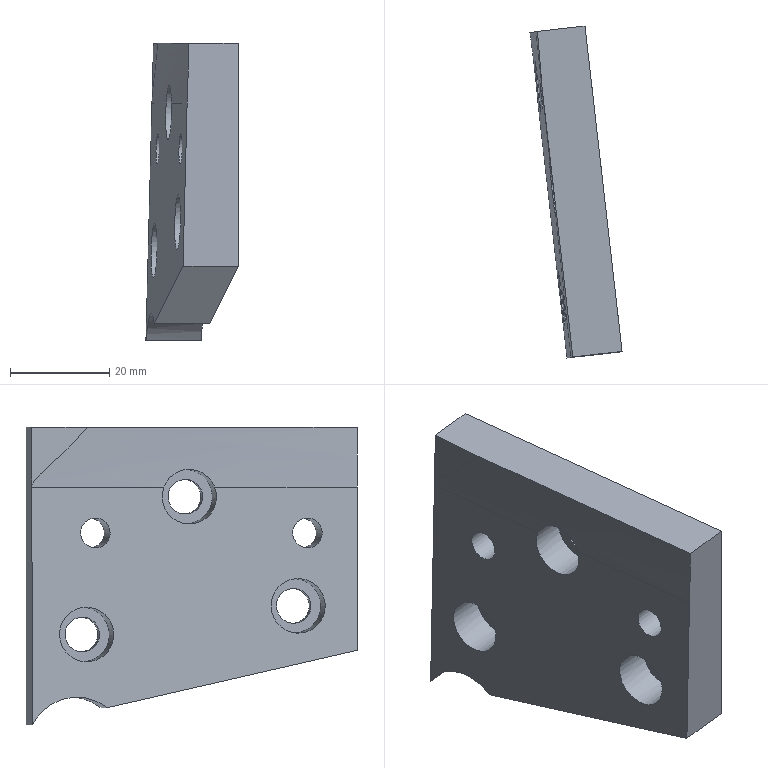Part | NX | features XQ 2 | 1 solid | 21 faces | box 18.578 x 66.841 x 59.998 mm | volume 32864 mm3 | plane 11 | cylinder 9 | spline 1 | commonest cylinder face diameters 7 x3 11 x3 6.001 x2 20 x1
STEP:
#1=CARTESIAN_POINT('',(2664.559,193.904,-66.597));
#2=VERTEX_POINT('',#1);
#3=CARTESIAN_POINT('',(2664.604,193.511,-63.12));
#4=DIRECTION('',(-0.9936,-0.1132,0.));
#5=DIRECTION('',(-0.01281,0.1125,-0.9936));
#6=AXIS2_PLACEMENT_3D('',#3,#4,#5);
#7=CIRCLE('',#6,3.5);
#8=EDGE_CURVE('',#2,#2,#7,.T.);
#9=ORIENTED_EDGE('',*,*,#8,.F.);
#10=EDGE_LOOP('',(#9));
#11=FACE_BOUND('',#10,.T.);
#12=CARTESIAN_POINT('',(2664.674,192.892,-57.655));
#13=VERTEX_POINT('',#12);
#14=CARTESIAN_POINT('',(2664.604,193.511,-63.12));
#15=DIRECTION('',(-0.9936,-0.1132,0.));
#16=DIRECTION('',(0.01281,-0.1125,0.9936));
#17=AXIS2_PLACEMENT_3D('',#14,#15,#16);
#18=CIRCLE('',#17,5.5);
#19=EDGE_CURVE('',#13,#13,#18,.T.);
#20=ORIENTED_EDGE('',*,*,#19,.T.);
#21=EDGE_LOOP('',(#20));
#22=FACE_BOUND('',#21,.T.);
#23=CARTESIAN_POINT('',(2664.604,193.511,-63.12));
#24=DIRECTION('',(0.9936,0.1132,0.));
#25=DIRECTION('',(0.01281,-0.1125,0.9936));
#26=AXIS2_PLACEMENT_3D('',#23,#24,#25);
#27=PLANE('',#26);
#28=ADVANCED_FACE('',(#11,#22),#27,.F.);
#29=CARTESIAN_POINT('',(2659.703,236.529,-72.371));
#30=VERTEX_POINT('',#29);
#31=CARTESIAN_POINT('',(2659.747,236.136,-68.894));
#32=DIRECTION('',(-0.9936,-0.1132,0.));
#33=DIRECTION('',(-0.01281,0.1125,-0.9936));
#34=AXIS2_PLACEMENT_3D('',#31,#32,#33);
#35=CIRCLE('',#34,3.5);
#36=EDGE_CURVE('',#30,#30,#35,.T.);
#37=ORIENTED_EDGE('',*,*,#36,.F.);
#38=EDGE_LOOP('',(#37));
#39=FACE_BOUND('',#38,.T.);
#40=CARTESIAN_POINT('',(2659.818,235.517,-63.429));
#41=VERTEX_POINT('',#40);
#42=CARTESIAN_POINT('',(2659.747,236.136,-68.894));
#43=DIRECTION('',(-0.9936,-0.1132,0.));
#44=DIRECTION('',(0.01281,-0.1125,0.9936));
#45=AXIS2_PLACEMENT_3D('',#42,#43,#44);
#46=CIRCLE('',#45,5.5);
#47=EDGE_CURVE('',#41,#41,#46,.T.);
#48=ORIENTED_EDGE('',*,*,#47,.T.);
#49=EDGE_LOOP('',(#48));
#50=FACE_BOUND('',#49,.T.);
#51=CARTESIAN_POINT('',(2659.747,236.136,-68.894));
#52=DIRECTION('',(0.9936,0.1132,0.));
#53=DIRECTION('',(0.01281,-0.1125,0.9936));
#54=AXIS2_PLACEMENT_3D('',#51,#52,#53);
#55=PLANE('',#54);
#56=ADVANCED_FACE('',(#39,#50),#55,.F.);
#57=CARTESIAN_POINT('',(2662.184,214.751,-35.655));
#58=VERTEX_POINT('',#57);
#59=CARTESIAN_POINT('',(2662.113,215.369,-41.12));
#60=DIRECTION('',(-0.9936,-0.1132,0.));
#61=DIRECTION('',(0.01281,-0.1125,0.9936));
#62=AXIS2_PLACEMENT_3D('',#59,#60,#61);
#63=CIRCLE('',#62,5.5);
#64=EDGE_CURVE('',#58,#58,#63,.T.);
#65=ORIENTED_EDGE('',*,*,#64,.T.);
#66=EDGE_LOOP('',(#65));
#67=FACE_BOUND('',#66,.T.);
#68=CARTESIAN_POINT('',(2662.069,215.763,-44.597));
#69=VERTEX_POINT('',#68);
#70=CARTESIAN_POINT('',(2662.113,215.369,-41.12));
#71=DIRECTION('',(-0.9936,-0.1132,0.));
#72=DIRECTION('',(-0.01281,0.1125,-0.9936));
#73=AXIS2_PLACEMENT_3D('',#70,#71,#72);
#74=CIRCLE('',#73,3.5);
#75=EDGE_CURVE('',#69,#69,#74,.T.);
#76=ORIENTED_EDGE('',*,*,#75,.F.);
#77=EDGE_LOOP('',(#76));
#78=FACE_BOUND('',#77,.T.);
#79=CARTESIAN_POINT('',(2662.113,215.369,-41.12));
#80=DIRECTION('',(0.9936,0.1132,0.));
#81=DIRECTION('',(0.01281,-0.1125,0.9936));
#82=AXIS2_PLACEMENT_3D('',#79,#80,#81);
#83=PLANE('',#82);
#84=ADVANCED_FACE('',(#67,#78),#83,.F.);
#85=ORIENTED_EDGE('',*,*,#19,.F.);
#86=EDGE_LOOP('',(#85));
#87=FACE_BOUND('',#86,.T.);
#88=CARTESIAN_POINT('',(2656.779,193.849,-57.757));
#89=VERTEX_POINT('',#88);
#90=CARTESIAN_POINT('',(2656.775,192.619,-63.12));
#91=DIRECTION('',(-0.9939,-0.1074,0.02552));
#92=DIRECTION('',(0.0008715,0.2236,0.9747));
#93=AXIS2_PLACEMENT_3D('',#90,#91,#92);
#94=ELLIPSE('',#93,5.502,5.5);
#95=EDGE_CURVE('',#89,#89,#94,.T.);
#96=ORIENTED_EDGE('',*,*,#95,.T.);
#97=EDGE_LOOP('',(#96));
#98=FACE_BOUND('',#97,.T.);
#99=CARTESIAN_POINT('',(2657.649,192.718,-63.12));
#100=DIRECTION('',(0.9936,0.1132,0.));
#101=DIRECTION('',(-0.01281,0.1125,-0.9936));
#102=AXIS2_PLACEMENT_3D('',#99,#100,#101);
#103=CYLINDRICAL_SURFACE('',#102,5.5);
#104=ADVANCED_FACE('',(#87,#98),#103,.F.);
#105=CARTESIAN_POINT('',(2667.981,190.373,-63.12));
#106=VERTEX_POINT('',#105);
#107=CARTESIAN_POINT('',(2667.585,193.85,-63.12));
#108=DIRECTION('',(-0.9936,-0.1132,-0.000000001));
#109=DIRECTION('',(0.1132,-0.9936,0.));
#110=AXIS2_PLACEMENT_3D('',#107,#108,#109);
#111=CIRCLE('',#110,3.5);
#112=EDGE_CURVE('',#106,#106,#111,.T.);
#113=ORIENTED_EDGE('',*,*,#112,.F.);
#114=EDGE_LOOP('',(#113));
#115=FACE_BOUND('',#114,.T.);
#116=ORIENTED_EDGE('',*,*,#8,.T.);
#117=EDGE_LOOP('',(#116));
#118=FACE_BOUND('',#117,.T.);
#119=CARTESIAN_POINT('',(2655.662,192.492,-63.12));
#120=DIRECTION('',(0.9936,0.1132,0.));
#121=DIRECTION('',(-0.01281,0.1125,-0.9936));
#122=AXIS2_PLACEMENT_3D('',#119,#120,#121);
#123=CYLINDRICAL_SURFACE('',#122,3.5);
#124=ADVANCED_FACE('',(#115,#118),#123,.F.);
#125=CARTESIAN_POINT('',(2668.142,188.959,-48.416));
#126=VERTEX_POINT('',#125);
#127=CARTESIAN_POINT('',(2667.802,191.94,-48.416));
#128=DIRECTION('',(-0.9936,-0.1132,-0.000000001));
#129=DIRECTION('',(0.1132,-0.9936,0.));
#130=AXIS2_PLACEMENT_3D('',#127,#128,#129);
#131=CIRCLE('',#130,3.001);
#132=EDGE_CURVE('',#126,#126,#131,.T.);
#133=ORIENTED_EDGE('',*,*,#132,.F.);
#134=EDGE_LOOP('',(#133));
#135=FACE_BOUND('',#134,.T.);
#136=CARTESIAN_POINT('',(2657.357,191.421,-45.49));
#137=VERTEX_POINT('',#136);
#138=CARTESIAN_POINT('',(2657.354,190.75,-48.416));
#139=DIRECTION('',(-0.9939,-0.1074,0.02552));
#140=DIRECTION('',(0.0008715,0.2236,0.9747));
#141=AXIS2_PLACEMENT_3D('',#138,#139,#140);
#142=ELLIPSE('',#141,3.002,3.001);
#143=EDGE_CURVE('',#137,#137,#142,.T.);
#144=ORIENTED_EDGE('',*,*,#143,.T.);
#145=EDGE_LOOP('',(#144));
#146=FACE_BOUND('',#145,.T.);
#147=CARTESIAN_POINT('',(2655.879,190.582,-48.416));
#148=DIRECTION('',(0.9936,0.1132,0.));
#149=DIRECTION('',(-0.01281,0.1125,-0.9936));
#150=AXIS2_PLACEMENT_3D('',#147,#148,#149);
#151=CYLINDRICAL_SURFACE('',#150,3.001);
#152=ADVANCED_FACE('',(#135,#146),#151,.F.);
#153=CARTESIAN_POINT('',(2658.679,180.692,-39.162));
#154=VERTEX_POINT('',#153);
#155=CARTESIAN_POINT('',(2657.844,180.597,-72.062));
#156=VERTEX_POINT('',#155);
#157=CARTESIAN_POINT('',(2659.681,180.806,0.3658));
#158=DIRECTION('',(-0.02536,-0.002889,-0.9997));
#159=VECTOR('',#158,1000.);
#160=LINE('',#157,#159);
#161=EDGE_CURVE('',#154,#156,#160,.T.);
#162=ORIENTED_EDGE('',*,*,#161,.T.);
#163=CARTESIAN_POINT('',(2668.95,181.863,-72.062));
#164=VERTEX_POINT('',#163);
#165=CARTESIAN_POINT('',(2673.918,182.429,-72.062));
#166=DIRECTION('',(-0.9936,-0.1132,-0.000000001));
#167=VECTOR('',#166,1000.);
#168=LINE('',#165,#167);
#169=EDGE_CURVE('',#164,#156,#168,.T.);
#170=ORIENTED_EDGE('',*,*,#169,.F.);
#171=CARTESIAN_POINT('',(2668.95,181.863,-27.1));
#172=VERTEX_POINT('',#171);
#173=CARTESIAN_POINT('',(2668.95,181.863,-0.000000058));
#174=DIRECTION('',(0.000000001,0.,-1.));
#175=VECTOR('',#174,1000.);
#176=LINE('',#173,#175);
#177=EDGE_CURVE('',#172,#164,#176,.T.);
#178=ORIENTED_EDGE('',*,*,#177,.F.);
#179=CARTESIAN_POINT('',(2659.015,180.73,-27.1));
#180=VERTEX_POINT('',#179);
#181=CARTESIAN_POINT('',(2673.918,182.429,-27.1));
#182=DIRECTION('',(0.9936,0.1132,0.));
#183=VECTOR('',#182,1000.);
#184=LINE('',#181,#183);
#185=EDGE_CURVE('',#180,#172,#184,.T.);
#186=ORIENTED_EDGE('',*,*,#185,.F.);
#187=CARTESIAN_POINT('',(2659.015,180.73,-27.1));
#188=CARTESIAN_POINT('',(2659.015,180.73,-31.123));
#189=CARTESIAN_POINT('',(2658.781,180.704,-35.141));
#190=CARTESIAN_POINT('',(2658.679,180.692,-39.162));
#191=B_SPLINE_CURVE_WITH_KNOTS('',3,(#187,#188,#189,#190),.UNSPECIFIED.,.F.,.F.,(4,4),(0.,0.01207),.UNSPECIFIED.);
#192=EDGE_CURVE('',#180,#154,#191,.T.);
#193=ORIENTED_EDGE('',*,*,#192,.T.);
#194=EDGE_LOOP('',(#162,#170,#178,#186,#193));
#195=FACE_BOUND('',#194,.T.);
#196=CARTESIAN_POINT('',(2673.918,182.429,-0.000000058));
#197=DIRECTION('',(0.1132,-0.9936,0.));
#198=DIRECTION('',(0.9936,0.1132,0.));
#199=AXIS2_PLACEMENT_3D('',#196,#197,#198);
#200=PLANE('',#199);
#201=ADVANCED_FACE('',(#195),#200,.T.);
#202=CARTESIAN_POINT('',(2652.091,231.089,-83.639));
#203=VERTEX_POINT('',#202);
#204=CARTESIAN_POINT('',(2663.198,232.355,-83.639));
#205=VERTEX_POINT('',#204);
#206=CARTESIAN_POINT('',(3040.755,275.372,-83.639));
#207=DIRECTION('',(0.9936,0.1132,0.000000001));
#208=VECTOR('',#207,1000.);
#209=LINE('',#206,#208);
#210=EDGE_CURVE('',#203,#205,#209,.T.);
#211=ORIENTED_EDGE('',*,*,#210,.T.);
#212=CARTESIAN_POINT('',(2503.911,1630.398,-404.205));
#213=DIRECTION('',(0.1104,-0.9687,0.2221));
#214=VECTOR('',#213,1000.);
#215=LINE('',#212,#214);
#216=EDGE_CURVE('',#205,#164,#215,.T.);
#217=ORIENTED_EDGE('',*,*,#216,.T.);
#218=ORIENTED_EDGE('',*,*,#169,.T.);
#219=CARTESIAN_POINT('',(2492.804,1629.133,-404.205));
#220=DIRECTION('',(0.1104,-0.9687,0.2221));
#221=VECTOR('',#220,1000.);
#222=LINE('',#219,#221);
#223=EDGE_CURVE('',#203,#156,#222,.T.);
#224=ORIENTED_EDGE('',*,*,#223,.F.);
#225=EDGE_LOOP('',(#211,#217,#218,#224));
#226=FACE_BOUND('',#225,.T.);
#227=CARTESIAN_POINT('',(2652.739,302.066,-99.689));
#228=DIRECTION('',(0.02515,-0.2207,-0.975));
#229=DIRECTION('',(0.,0.9753,-0.2208));
#230=AXIS2_PLACEMENT_3D('',#227,#228,#229);
#231=PLANE('',#230);
#232=ADVANCED_FACE('',(#226),#231,.T.);
#233=CARTESIAN_POINT('',(2661.482,247.415,-87.093));
#234=VERTEX_POINT('',#233);
#235=CARTESIAN_POINT('',(2662.498,238.496,-91.5));
#236=DIRECTION('',(-0.9936,-0.1132,-0.000000001));
#237=DIRECTION('',(0.000000001,0.,-1.));
#238=AXIS2_PLACEMENT_3D('',#235,#236,#237);
#239=CIRCLE('',#238,10.);
#240=EDGE_CURVE('',#205,#234,#239,.T.);
#241=ORIENTED_EDGE('',*,*,#240,.F.);
#242=ORIENTED_EDGE('',*,*,#210,.F.);
#243=CARTESIAN_POINT('',(2650.375,246.149,-87.093));
#244=VERTEX_POINT('',#243);
#245=CARTESIAN_POINT('',(2651.228,237.212,-91.5));
#246=DIRECTION('',(-0.9939,-0.1074,0.02552));
#247=DIRECTION('',(-0.0008715,-0.2236,-0.9747));
#248=AXIS2_PLACEMENT_3D('',#245,#246,#247);
#249=ELLIPSE('',#248,10.003,10.);
#250=EDGE_CURVE('',#203,#244,#249,.T.);
#251=ORIENTED_EDGE('',*,*,#250,.T.);
#252=CARTESIAN_POINT('',(3039.039,290.432,-87.093));
#253=DIRECTION('',(-0.9936,-0.1132,-0.000000001));
#254=VECTOR('',#253,1000.);
#255=LINE('',#252,#254);
#256=EDGE_CURVE('',#234,#244,#255,.T.);
#257=ORIENTED_EDGE('',*,*,#256,.F.);
#258=EDGE_LOOP('',(#241,#242,#251,#257));
#259=FACE_BOUND('',#258,.T.);
#260=CARTESIAN_POINT('',(3040.055,281.513,-91.5));
#261=DIRECTION('',(-0.9936,-0.1132,-0.000000001));
#262=DIRECTION('',(0.000000001,0.,-1.));
#263=AXIS2_PLACEMENT_3D('',#260,#261,#262);
#264=CYLINDRICAL_SURFACE('',#263,10.);
#265=ADVANCED_FACE('',(#259),#264,.F.);
#266=CARTESIAN_POINT('',(2650.373,246.173,-87.098));
#267=VERTEX_POINT('',#266);
#268=CARTESIAN_POINT('',(2661.479,247.438,-87.098));
#269=VERTEX_POINT('',#268);
#270=CARTESIAN_POINT('',(2658.995,247.155,-87.098));
#271=DIRECTION('',(0.9936,0.1132,0.000000001));
#272=VECTOR('',#271,1000.);
#273=LINE('',#270,#272);
#274=EDGE_CURVE('',#267,#269,#273,.T.);
#275=ORIENTED_EDGE('',*,*,#274,.T.);
#276=CARTESIAN_POINT('',(2503.911,1630.398,-404.205));
#277=DIRECTION('',(0.1104,-0.9687,0.2221));
#278=VECTOR('',#277,1000.);
#279=LINE('',#276,#278);
#280=EDGE_CURVE('',#269,#234,#279,.T.);
#281=ORIENTED_EDGE('',*,*,#280,.T.);
#282=ORIENTED_EDGE('',*,*,#256,.T.);
#283=CARTESIAN_POINT('',(2492.804,1629.133,-404.205));
#284=DIRECTION('',(0.1104,-0.9687,0.2221));
#285=VECTOR('',#284,1000.);
#286=LINE('',#283,#285);
#287=EDGE_CURVE('',#267,#244,#286,.T.);
#288=ORIENTED_EDGE('',*,*,#287,.F.);
#289=EDGE_LOOP('',(#275,#281,#282,#288));
#290=FACE_BOUND('',#289,.T.);
#291=CARTESIAN_POINT('',(2652.739,302.066,-99.689));
#292=DIRECTION('',(0.02515,-0.2207,-0.975));
#293=DIRECTION('',(0.,0.9753,-0.2208));
#294=AXIS2_PLACEMENT_3D('',#291,#292,#293);
#295=PLANE('',#294);
#296=ADVANCED_FACE('',(#290),#295,.T.);
#297=CARTESIAN_POINT('',(2651.895,246.346,-27.1));
#298=VERTEX_POINT('',#297);
#299=CARTESIAN_POINT('',(2651.593,246.312,-38.979));
#300=VERTEX_POINT('',#299);
#301=CARTESIAN_POINT('',(2651.895,246.346,-27.1));
#302=DIRECTION('',(-0.02539,-0.002893,-0.9997));
#303=VECTOR('',#302,1000.);
#304=LINE('',#301,#303);
#305=EDGE_CURVE('',#298,#300,#304,.T.);
#306=ORIENTED_EDGE('',*,*,#305,.F.);
#307=CARTESIAN_POINT('',(2661.479,247.438,-27.1));
#308=VERTEX_POINT('',#307);
#309=CARTESIAN_POINT('',(2651.543,246.306,-27.1));
#310=DIRECTION('',(0.9936,0.1132,0.));
#311=VECTOR('',#310,1000.);
#312=LINE('',#309,#311);
#313=EDGE_CURVE('',#298,#308,#312,.T.);
#314=ORIENTED_EDGE('',*,*,#313,.T.);
#315=CARTESIAN_POINT('',(2661.479,247.438,-706.6));
#316=DIRECTION('',(0.000000001,0.,-1.));
#317=VECTOR('',#316,1000.);
#318=LINE('',#315,#317);
#319=EDGE_CURVE('',#308,#269,#318,.T.);
#320=ORIENTED_EDGE('',*,*,#319,.T.);
#321=ORIENTED_EDGE('',*,*,#274,.F.);
#322=CARTESIAN_POINT('',(2651.588,246.311,-39.167));
#323=VERTEX_POINT('',#322);
#324=CARTESIAN_POINT('',(2651.328,246.282,-49.448));
#325=DIRECTION('',(-0.02536,-0.002889,-0.9997));
#326=VECTOR('',#325,1000.);
#327=LINE('',#324,#326);
#328=EDGE_CURVE('',#323,#267,#327,.T.);
#329=ORIENTED_EDGE('',*,*,#328,.F.);
#330=CARTESIAN_POINT('',(2651.593,246.312,-38.979));
#331=CARTESIAN_POINT('',(2651.591,246.312,-39.042));
#332=CARTESIAN_POINT('',(2651.59,246.312,-39.104));
#333=CARTESIAN_POINT('',(2651.588,246.311,-39.167));
#334=B_SPLINE_CURVE_WITH_KNOTS('',3,(#330,#331,#332,#333),.UNSPECIFIED.,.F.,.F.,(4,4),(0.,1.),.PIECEWISE_BEZIER_KNOTS.);
#335=EDGE_CURVE('',#300,#323,#334,.T.);
#336=ORIENTED_EDGE('',*,*,#335,.F.);
#337=EDGE_LOOP('',(#306,#314,#320,#321,#329,#336));
#338=FACE_BOUND('',#337,.T.);
#339=CARTESIAN_POINT('',(2656.511,246.872,-49.581));
#340=DIRECTION('',(0.1132,-0.9936,0.));
#341=DIRECTION('',(0.9936,0.1132,0.));
#342=AXIS2_PLACEMENT_3D('',#339,#340,#341);
#343=PLANE('',#342);
#344=ADVANCED_FACE('',(#338),#343,.F.);
#345=CARTESIAN_POINT('',(2663.124,232.998,-68.894));
#346=VERTEX_POINT('',#345);
#347=CARTESIAN_POINT('',(2662.728,236.475,-68.894));
#348=DIRECTION('',(-0.9936,-0.1132,-0.000000001));
#349=DIRECTION('',(0.1132,-0.9936,0.));
#350=AXIS2_PLACEMENT_3D('',#347,#348,#349);
#351=CIRCLE('',#350,3.5);
#352=EDGE_CURVE('',#346,#346,#351,.T.);
#353=ORIENTED_EDGE('',*,*,#352,.F.);
#354=EDGE_LOOP('',(#353));
#355=FACE_BOUND('',#354,.T.);
#356=ORIENTED_EDGE('',*,*,#36,.T.);
#357=EDGE_LOOP('',(#356));
#358=FACE_BOUND('',#357,.T.);
#359=CARTESIAN_POINT('',(2650.805,235.117,-68.894));
#360=DIRECTION('',(0.9936,0.1132,0.));
#361=DIRECTION('',(-0.01281,0.1125,-0.9936));
#362=AXIS2_PLACEMENT_3D('',#359,#360,#361);
#363=CYLINDRICAL_SURFACE('',#362,3.5);
#364=ADVANCED_FACE('',(#355,#358),#363,.F.);
#365=ORIENTED_EDGE('',*,*,#75,.T.);
#366=EDGE_LOOP('',(#365));
#367=FACE_BOUND('',#366,.T.);
#368=CARTESIAN_POINT('',(2665.49,212.231,-41.12));
#369=VERTEX_POINT('',#368);
#370=CARTESIAN_POINT('',(2665.094,215.709,-41.12));
#371=DIRECTION('',(-0.9936,-0.1132,-0.000000001));
#372=DIRECTION('',(0.1132,-0.9936,0.));
#373=AXIS2_PLACEMENT_3D('',#370,#371,#372);
#374=CIRCLE('',#373,3.5);
#375=EDGE_CURVE('',#369,#369,#374,.T.);
#376=ORIENTED_EDGE('',*,*,#375,.F.);
#377=EDGE_LOOP('',(#376));
#378=FACE_BOUND('',#377,.T.);
#379=CARTESIAN_POINT('',(2653.171,214.35,-41.12));
#380=DIRECTION('',(0.9936,0.1132,0.));
#381=DIRECTION('',(-0.01281,0.1125,-0.9936));
#382=AXIS2_PLACEMENT_3D('',#379,#380,#381);
#383=CYLINDRICAL_SURFACE('',#382,3.5);
#384=ADVANCED_FACE('',(#367,#378),#383,.F.);
#385=CARTESIAN_POINT('',(2511.71,1561.949,-27.1));
#386=DIRECTION('',(-0.1132,0.9936,0.));
#387=VECTOR('',#386,1000.);
#388=LINE('',#385,#387);
#389=EDGE_CURVE('',#172,#308,#388,.T.);
#390=ORIENTED_EDGE('',*,*,#389,.F.);
#391=ORIENTED_EDGE('',*,*,#177,.T.);
#392=ORIENTED_EDGE('',*,*,#216,.F.);
#393=ORIENTED_EDGE('',*,*,#240,.T.);
#394=ORIENTED_EDGE('',*,*,#280,.F.);
#395=ORIENTED_EDGE('',*,*,#319,.F.);
#396=EDGE_LOOP('',(#390,#391,#392,#393,#394,#395));
#397=FACE_BOUND('',#396,.T.);
#398=ORIENTED_EDGE('',*,*,#375,.T.);
#399=EDGE_LOOP('',(#398));
#400=FACE_BOUND('',#399,.T.);
#401=CARTESIAN_POINT('',(2663.274,231.683,-48.416));
#402=VERTEX_POINT('',#401);
#403=CARTESIAN_POINT('',(2662.934,234.664,-48.416));
#404=DIRECTION('',(-0.9936,-0.1132,-0.000000001));
#405=DIRECTION('',(0.1132,-0.9936,0.));
#406=AXIS2_PLACEMENT_3D('',#403,#404,#405);
#407=CIRCLE('',#406,3.001);
#408=EDGE_CURVE('',#402,#402,#407,.T.);
#409=ORIENTED_EDGE('',*,*,#408,.T.);
#410=EDGE_LOOP('',(#409));
#411=FACE_BOUND('',#410,.T.);
#412=ORIENTED_EDGE('',*,*,#352,.T.);
#413=EDGE_LOOP('',(#412));
#414=FACE_BOUND('',#413,.T.);
#415=ORIENTED_EDGE('',*,*,#132,.T.);
#416=EDGE_LOOP('',(#415));
#417=FACE_BOUND('',#416,.T.);
#418=ORIENTED_EDGE('',*,*,#112,.T.);
#419=EDGE_LOOP('',(#418));
#420=FACE_BOUND('',#419,.T.);
#421=CARTESIAN_POINT('',(2511.71,1561.949,-706.6));
#422=DIRECTION('',(0.9936,0.1132,0.000000001));
#423=DIRECTION('',(0.000000001,-0.000000001,-1.));
#424=AXIS2_PLACEMENT_3D('',#421,#422,#423);
#425=PLANE('',#424);
#426=ADVANCED_FACE('',(#397,#400,#411,#414,#417,#420),#425,.T.);
#427=ORIENTED_EDGE('',*,*,#47,.F.);
#428=EDGE_LOOP('',(#427));
#429=FACE_BOUND('',#428,.T.);
#430=CARTESIAN_POINT('',(2652.024,236.485,-63.531));
#431=VERTEX_POINT('',#430);
#432=CARTESIAN_POINT('',(2652.02,235.255,-68.894));
#433=DIRECTION('',(-0.9939,-0.1074,0.02552));
#434=DIRECTION('',(0.0008715,0.2236,0.9747));
#435=AXIS2_PLACEMENT_3D('',#432,#433,#434);
#436=ELLIPSE('',#435,5.502,5.5);
#437=EDGE_CURVE('',#431,#431,#436,.T.);
#438=ORIENTED_EDGE('',*,*,#437,.T.);
#439=EDGE_LOOP('',(#438));
#440=FACE_BOUND('',#439,.T.);
#441=CARTESIAN_POINT('',(2652.792,235.343,-68.894));
#442=DIRECTION('',(0.9936,0.1132,0.));
#443=DIRECTION('',(-0.01281,0.1125,-0.9936));
#444=AXIS2_PLACEMENT_3D('',#441,#442,#443);
#445=CYLINDRICAL_SURFACE('',#444,5.5);
#446=ADVANCED_FACE('',(#429,#440),#445,.F.);
#447=ORIENTED_EDGE('',*,*,#64,.F.);
#448=EDGE_LOOP('',(#447));
#449=FACE_BOUND('',#448,.T.);
#450=CARTESIAN_POINT('',(2655.571,209.45,-39.164));
#451=VERTEX_POINT('',#450);
#452=CARTESIAN_POINT('',(2654.467,219.672,-39.165));
#453=VERTEX_POINT('',#452);
#454=CARTESIAN_POINT('',(2655.571,209.45,-39.164));
#455=CARTESIAN_POINT('',(2655.555,209.848,-38.12));
#456=CARTESIAN_POINT('',(2655.451,211.266,-36.316));
#457=CARTESIAN_POINT('',(2655.108,214.569,-35.272));
#458=CARTESIAN_POINT('',(2654.729,217.868,-36.313));
#459=CARTESIAN_POINT('',(2654.536,219.28,-38.121));
#460=CARTESIAN_POINT('',(2654.467,219.672,-39.165));
#461=B_SPLINE_CURVE_WITH_KNOTS('',3,(#454,#455,#456,#457,#458,#459,#460),.UNSPECIFIED.,.F.,.F.,(4,1,1,1,4),(0.,0.003304,0.006608,0.009912,0.01322),.UNSPECIFIED.);
#462=EDGE_CURVE('',#451,#453,#461,.T.);
#463=ORIENTED_EDGE('',*,*,#462,.T.);
#464=CARTESIAN_POINT('',(2654.969,214.555,-41.12));
#465=DIRECTION('',(-0.9939,-0.1074,0.02552));
#466=DIRECTION('',(0.0008715,0.2236,0.9747));
#467=AXIS2_PLACEMENT_3D('',#464,#465,#466);
#468=ELLIPSE('',#467,5.502,5.5);
#469=EDGE_CURVE('',#453,#451,#468,.T.);
#470=ORIENTED_EDGE('',*,*,#469,.T.);
#471=EDGE_LOOP('',(#463,#470));
#472=FACE_BOUND('',#471,.T.);
#473=CARTESIAN_POINT('',(2655.158,214.577,-41.12));
#474=DIRECTION('',(0.9936,0.1132,0.));
#475=DIRECTION('',(-0.01281,0.1125,-0.9936));
#476=AXIS2_PLACEMENT_3D('',#473,#474,#475);
#477=CYLINDRICAL_SURFACE('',#476,5.5);
#478=ADVANCED_FACE('',(#449,#472),#477,.F.);
#479=CARTESIAN_POINT('',(2652.738,234.173,-45.49));
#480=VERTEX_POINT('',#479);
#481=CARTESIAN_POINT('',(2652.735,233.502,-48.416));
#482=DIRECTION('',(-0.9939,-0.1074,0.02552));
#483=DIRECTION('',(0.0008715,0.2236,0.9747));
#484=AXIS2_PLACEMENT_3D('',#481,#482,#483);
#485=ELLIPSE('',#484,3.002,3.001);
#486=EDGE_CURVE('',#480,#480,#485,.T.);
#487=ORIENTED_EDGE('',*,*,#486,.F.);
#488=EDGE_LOOP('',(#487));
#489=FACE_BOUND('',#488,.T.);
#490=ORIENTED_EDGE('',*,*,#328,.T.);
#491=ORIENTED_EDGE('',*,*,#287,.T.);
#492=ORIENTED_EDGE('',*,*,#250,.F.);
#493=ORIENTED_EDGE('',*,*,#223,.T.);
#494=ORIENTED_EDGE('',*,*,#161,.F.);
#495=CARTESIAN_POINT('',(2509.465,1561.67,-39.265));
#496=DIRECTION('',(-0.1074,0.9942,-0.00007422));
#497=VECTOR('',#496,1000.);
#498=LINE('',#495,#497);
#499=EDGE_CURVE('',#154,#451,#498,.T.);
#500=ORIENTED_EDGE('',*,*,#499,.T.);
#501=ORIENTED_EDGE('',*,*,#469,.F.);
#502=CARTESIAN_POINT('',(2509.465,1561.67,-39.265));
#503=DIRECTION('',(-0.1074,0.9942,-0.00007422));
#504=VECTOR('',#503,1000.);
#505=LINE('',#502,#504);
#506=EDGE_CURVE('',#453,#323,#505,.T.);
#507=ORIENTED_EDGE('',*,*,#506,.T.);
#508=EDGE_LOOP('',(#490,#491,#492,#493,#494,#500,#501,#507));
#509=FACE_BOUND('',#508,.T.);
#510=ORIENTED_EDGE('',*,*,#437,.F.);
#511=EDGE_LOOP('',(#510));
#512=FACE_BOUND('',#511,.T.);
#513=ORIENTED_EDGE('',*,*,#143,.F.);
#514=EDGE_LOOP('',(#513));
#515=FACE_BOUND('',#514,.T.);
#516=ORIENTED_EDGE('',*,*,#95,.F.);
#517=EDGE_LOOP('',(#516));
#518=FACE_BOUND('',#517,.T.);
#519=CARTESIAN_POINT('',(2492.534,1559.791,-706.481));
#520=DIRECTION('',(0.9939,0.1074,-0.02552));
#521=DIRECTION('',(-0.02537,-0.002816,-0.9997));
#522=AXIS2_PLACEMENT_3D('',#519,#520,#521);
#523=PLANE('',#522);
#524=ADVANCED_FACE('',(#489,#509,#512,#515,#518),#523,.F.);
#525=ORIENTED_EDGE('',*,*,#408,.F.);
#526=EDGE_LOOP('',(#525));
#527=FACE_BOUND('',#526,.T.);
#528=ORIENTED_EDGE('',*,*,#486,.T.);
#529=EDGE_LOOP('',(#528));
#530=FACE_BOUND('',#529,.T.);
#531=CARTESIAN_POINT('',(2651.012,233.306,-48.416));
#532=DIRECTION('',(0.9936,0.1132,0.));
#533=DIRECTION('',(-0.01281,0.1125,-0.9936));
#534=AXIS2_PLACEMENT_3D('',#531,#532,#533);
#535=CYLINDRICAL_SURFACE('',#534,3.001);
#536=ADVANCED_FACE('',(#527,#530),#535,.F.);
#537=CARTESIAN_POINT('',(2652.816,235.132,-27.1));
#538=VERTEX_POINT('',#537);
#539=CARTESIAN_POINT('',(2655.596,201.327,-27.1));
#540=DIRECTION('',(0.08193,-0.9966,0.));
#541=VECTOR('',#540,1000.);
#542=LINE('',#539,#541);
#543=EDGE_CURVE('',#298,#538,#542,.T.);
#544=ORIENTED_EDGE('',*,*,#543,.T.);
#545=CARTESIAN_POINT('',(2659.015,180.73,-27.1));
#546=CARTESIAN_POINT('',(2657.974,189.868,-27.1));
#547=CARTESIAN_POINT('',(2656.933,199.006,-27.1));
#548=CARTESIAN_POINT('',(2654.866,217.14,-27.1));
#549=CARTESIAN_POINT('',(2653.841,226.136,-27.1));
#550=CARTESIAN_POINT('',(2652.816,235.132,-27.1));
#551=B_SPLINE_CURVE_WITH_KNOTS('',3,(#545,#546,#547,#548,#549,#550),.UNSPECIFIED.,.F.,.F.,(4,2,4),(0.,0.5039,1.),.UNSPECIFIED.);
#552=EDGE_CURVE('',#180,#538,#551,.T.);
#553=ORIENTED_EDGE('',*,*,#552,.F.);
#554=ORIENTED_EDGE('',*,*,#185,.T.);
#555=ORIENTED_EDGE('',*,*,#389,.T.);
#556=ORIENTED_EDGE('',*,*,#313,.F.);
#557=EDGE_LOOP('',(#544,#553,#554,#555,#556));
#558=FACE_BOUND('',#557,.T.);
#559=CARTESIAN_POINT('',(2656.658,201.414,-27.1));
#560=DIRECTION('',(0.,0.,1.));
#561=DIRECTION('',(-1.,0.,0.));
#562=AXIS2_PLACEMENT_3D('',#559,#560,#561);
#563=PLANE('',#562);
#564=ADVANCED_FACE('',(#558),#563,.T.);
#565=ORIENTED_EDGE('',*,*,#506,.F.);
#566=ORIENTED_EDGE('',*,*,#462,.F.);
#567=ORIENTED_EDGE('',*,*,#499,.F.);
#568=ORIENTED_EDGE('',*,*,#192,.F.);
#569=ORIENTED_EDGE('',*,*,#552,.T.);
#570=CARTESIAN_POINT('',(2651.593,246.31,-38.978));
#571=VERTEX_POINT('',#570);
#572=CARTESIAN_POINT('',(2651.593,246.31,-38.978));
#573=CARTESIAN_POINT('',(2651.599,246.287,-38.83));
#574=CARTESIAN_POINT('',(2651.613,246.206,-38.539));
#575=CARTESIAN_POINT('',(2651.645,245.954,-38.103));
#576=CARTESIAN_POINT('',(2651.665,245.781,-37.867));
#577=CARTESIAN_POINT('',(2651.688,245.579,-37.619));
#578=CARTESIAN_POINT('',(2651.7,245.471,-37.496));
#579=CARTESIAN_POINT('',(2651.734,245.162,-37.151));
#580=CARTESIAN_POINT('',(2651.758,244.946,-36.922));
#581=CARTESIAN_POINT('',(2651.805,244.51,-36.482));
#582=CARTESIAN_POINT('',(2651.833,244.247,-36.23));
#583=CARTESIAN_POINT('',(2651.886,243.75,-35.761));
#584=CARTESIAN_POINT('',(2651.909,243.535,-35.562));
#585=CARTESIAN_POINT('',(2651.96,243.054,-35.118));
#586=CARTESIAN_POINT('',(2652.04,242.293,-34.425));
#587=CARTESIAN_POINT('',(2652.124,241.502,-33.703));
#588=CARTESIAN_POINT('',(2652.174,241.029,-33.268));
#589=CARTESIAN_POINT('',(2652.196,240.817,-33.072));
#590=CARTESIAN_POINT('',(2652.245,240.359,-32.643));
#591=CARTESIAN_POINT('',(2652.299,239.852,-32.162));
#592=CARTESIAN_POINT('',(2652.366,239.218,-31.55));
#593=CARTESIAN_POINT('',(2652.444,238.5,-30.836));
#594=CARTESIAN_POINT('',(2652.512,237.873,-30.196));
#595=CARTESIAN_POINT('',(2652.596,237.101,-29.379));
#596=CARTESIAN_POINT('',(2652.698,236.184,-28.364));
#597=CARTESIAN_POINT('',(2652.77,235.537,-27.601));
#598=CARTESIAN_POINT('',(2652.816,235.132,-27.1));
#599=B_SPLINE_CURVE_WITH_KNOTS('',3,(#572,#573,#574,#575,#576,#577,#578,#579,#580,#581,#582,#583,#584,#585,#586,#587,#588,#589,#590,#591,#592,#593,#594,#595,#596,#597,#598),.UNSPECIFIED.,.F.,.F.,(4,1,1,1,1,1,1,1,1,1,1,1,1,1,1,1,1,1,1,1,1,1,1,1,4),(0.,0.03125,0.0625,0.07812,0.09375,0.1094,0.125,0.1562,0.1875,0.2188,0.25,0.2812,0.3125,0.375,0.4375,0.4688,0.5,0.5312,0.5625,0.625,0.6875,0.75,0.8125,0.875,1.),.UNSPECIFIED.);
#600=EDGE_CURVE('',#571,#538,#599,.T.);
#601=ORIENTED_EDGE('',*,*,#600,.F.);
#602=CARTESIAN_POINT('',(2651.593,246.312,-38.979));
#603=CARTESIAN_POINT('',(2651.593,246.311,-38.978));
#604=CARTESIAN_POINT('',(2651.593,246.31,-38.978));
#605=CARTESIAN_POINT('',(2651.593,246.31,-38.978));
#606=B_SPLINE_CURVE_WITH_KNOTS('',3,(#602,#603,#604,#605),.UNSPECIFIED.,.F.,.F.,(4,4),(0.,1.),.UNSPECIFIED.);
#607=EDGE_CURVE('',#300,#571,#606,.T.);
#608=ORIENTED_EDGE('',*,*,#607,.F.);
#609=ORIENTED_EDGE('',*,*,#335,.T.);
#610=EDGE_LOOP('',(#565,#566,#567,#568,#569,#601,#608,#609));
#611=FACE_BOUND('',#610,.T.);
#612=CARTESIAN_POINT('',(2659.049,180.426,-27.035));
#613=CARTESIAN_POINT('',(2656.966,198.71,-27.013));
#614=CARTESIAN_POINT('',(2654.883,216.995,-26.992));
#615=CARTESIAN_POINT('',(2652.8,235.279,-26.971));
#616=CARTESIAN_POINT('',(2659.05,180.419,-27.056));
#617=CARTESIAN_POINT('',(2656.964,198.725,-27.042));
#618=CARTESIAN_POINT('',(2654.879,217.032,-27.028));
#619=CARTESIAN_POINT('',(2652.793,235.339,-27.014));
#620=CARTESIAN_POINT('',(2659.086,180.108,-27.987));
#621=CARTESIAN_POINT('',(2656.892,199.367,-28.276));
#622=CARTESIAN_POINT('',(2654.697,218.626,-28.564));
#623=CARTESIAN_POINT('',(2652.503,237.885,-28.852));
#624=CARTESIAN_POINT('',(2659.13,179.448,-29.871));
#625=CARTESIAN_POINT('',(2656.722,200.719,-30.624));
#626=CARTESIAN_POINT('',(2654.314,221.99,-31.377));
#627=CARTESIAN_POINT('',(2651.906,243.261,-32.131));
#628=CARTESIAN_POINT('',(2659.151,178.362,-32.802));
#629=CARTESIAN_POINT('',(2656.42,202.932,-33.814));
#630=CARTESIAN_POINT('',(2653.688,227.502,-34.826));
#631=CARTESIAN_POINT('',(2650.957,252.073,-35.838));
#632=CARTESIAN_POINT('',(2659.158,177.19,-35.886));
#633=CARTESIAN_POINT('',(2656.086,205.314,-36.687));
#634=CARTESIAN_POINT('',(2653.014,233.438,-37.488));
#635=CARTESIAN_POINT('',(2649.943,261.563,-38.289));
#636=CARTESIAN_POINT('',(2659.174,176.369,-38.051));
#637=CARTESIAN_POINT('',(2655.858,206.987,-38.377));
#638=CARTESIAN_POINT('',(2652.541,237.605,-38.704));
#639=CARTESIAN_POINT('',(2649.224,268.223,-39.03));
#640=CARTESIAN_POINT('',(2659.191,175.953,-39.162));
#641=CARTESIAN_POINT('',(2655.746,207.837,-39.164));
#642=CARTESIAN_POINT('',(2652.301,239.721,-39.166));
#643=CARTESIAN_POINT('',(2648.855,271.605,-39.169));
#644=B_SPLINE_SURFACE_WITH_KNOTS('',3,3,((#612,#613,#614,#615),(#616,#617,#618,#619),(#620,#621,#622,#623),(#624,#625,#626,#627),(#628,#629,#630,#631),(#632,#633,#634,#635),(#636,#637,#638,#639),(#640,#641,#642,#643)),.RULED_SURF.,.F.,.F.,.F.,(4,1,1,1,1,4),(4,4),(0.,0.005964,0.2545,0.503,0.7515,1.),(0.2727,0.8299),.UNSPECIFIED.);
#645=ADVANCED_FACE('',(#611),#644,.F.);
#646=ORIENTED_EDGE('',*,*,#543,.F.);
#647=ORIENTED_EDGE('',*,*,#305,.T.);
#648=ORIENTED_EDGE('',*,*,#607,.T.);
#649=ORIENTED_EDGE('',*,*,#600,.T.);
#650=EDGE_LOOP('',(#646,#647,#648,#649));
#651=FACE_BOUND('',#650,.T.);
#652=CARTESIAN_POINT('',(2651.895,246.346,-27.1));
#653=DIRECTION('',(0.9963,0.08191,-0.02554));
#654=DIRECTION('',(-0.08193,0.9966,0.));
#655=AXIS2_PLACEMENT_3D('',#652,#653,#654);
#656=PLANE('',#655);
#657=ADVANCED_FACE('',(#651),#656,.F.);
#658=CLOSED_SHELL('',(#28,#56,#84,#104,#124,#152,#201,#232,#265,#296,#344,#364,#384,#426,#446,#478,#524,#536,#564,#645,#657));
#659=MANIFOLD_SOLID_BREP('',#658);
#660=(LENGTH_UNIT()NAMED_UNIT(*)SI_UNIT(.MILLI.,.METRE.));
#661=UNCERTAINTY_MEASURE_WITH_UNIT(LENGTH_MEASURE(0.0508),#660,'','');
#662=(NAMED_UNIT(*)PLANE_ANGLE_UNIT()SI_UNIT($,.RADIAN.));
#663=(NAMED_UNIT(*)SI_UNIT($,.STERADIAN.)SOLID_ANGLE_UNIT());
#664=(GEOMETRIC_REPRESENTATION_CONTEXT(3)GLOBAL_UNCERTAINTY_ASSIGNED_CONTEXT((#661))GLOBAL_UNIT_ASSIGNED_CONTEXT((#660,#662,#663))REPRESENTATION_CONTEXT('',''));
#665=ADVANCED_BREP_SHAPE_REPRESENTATION('',(#659),#664);